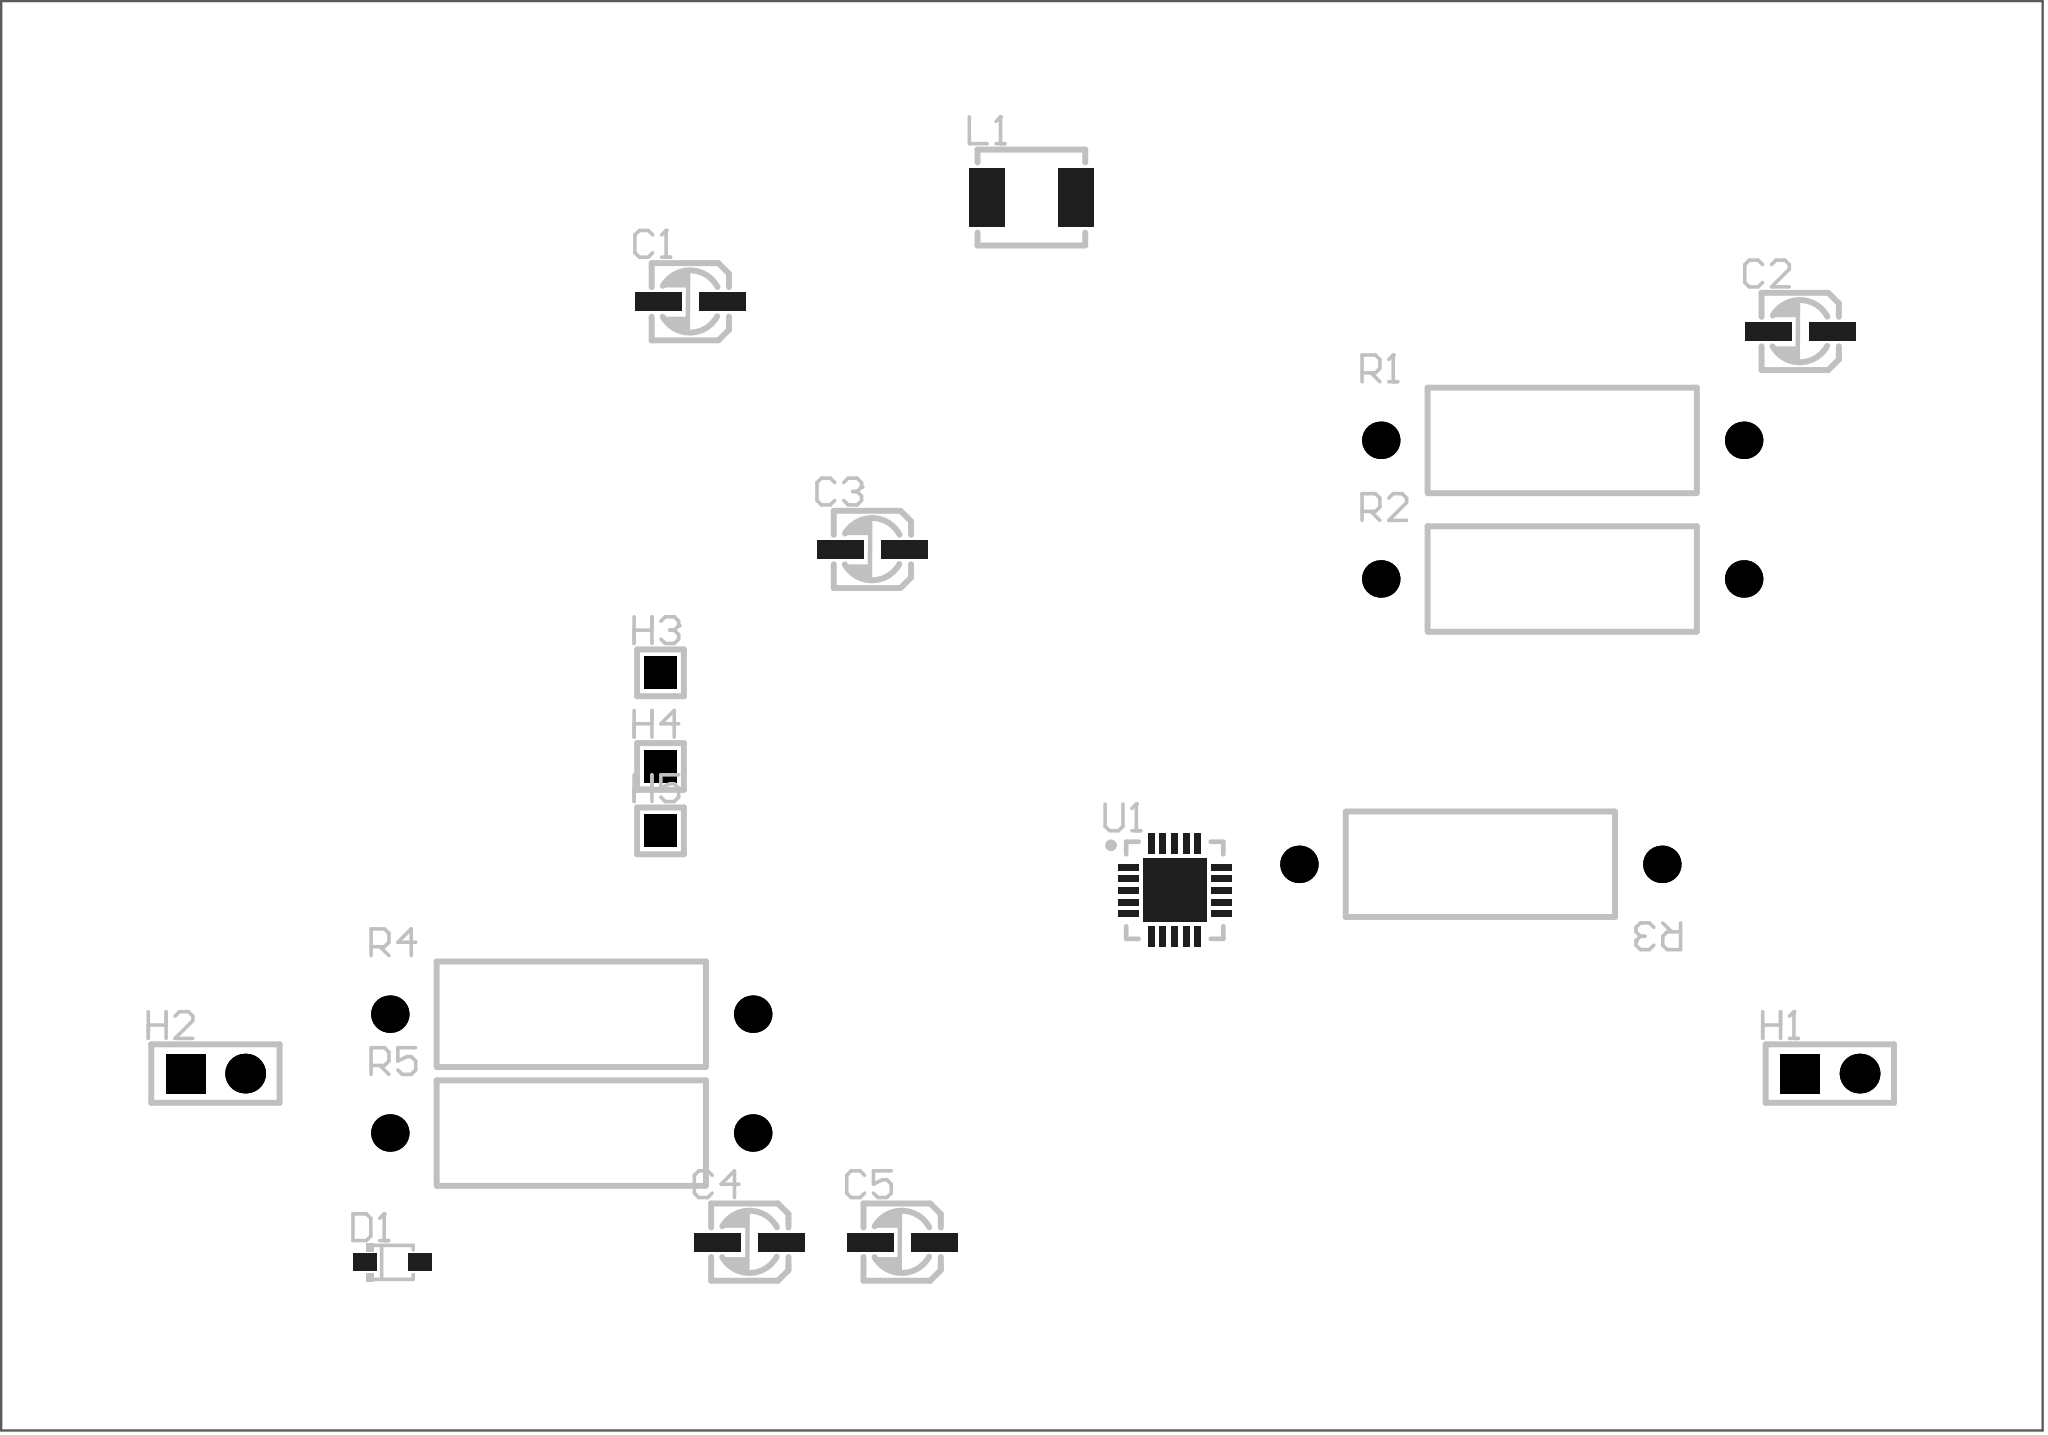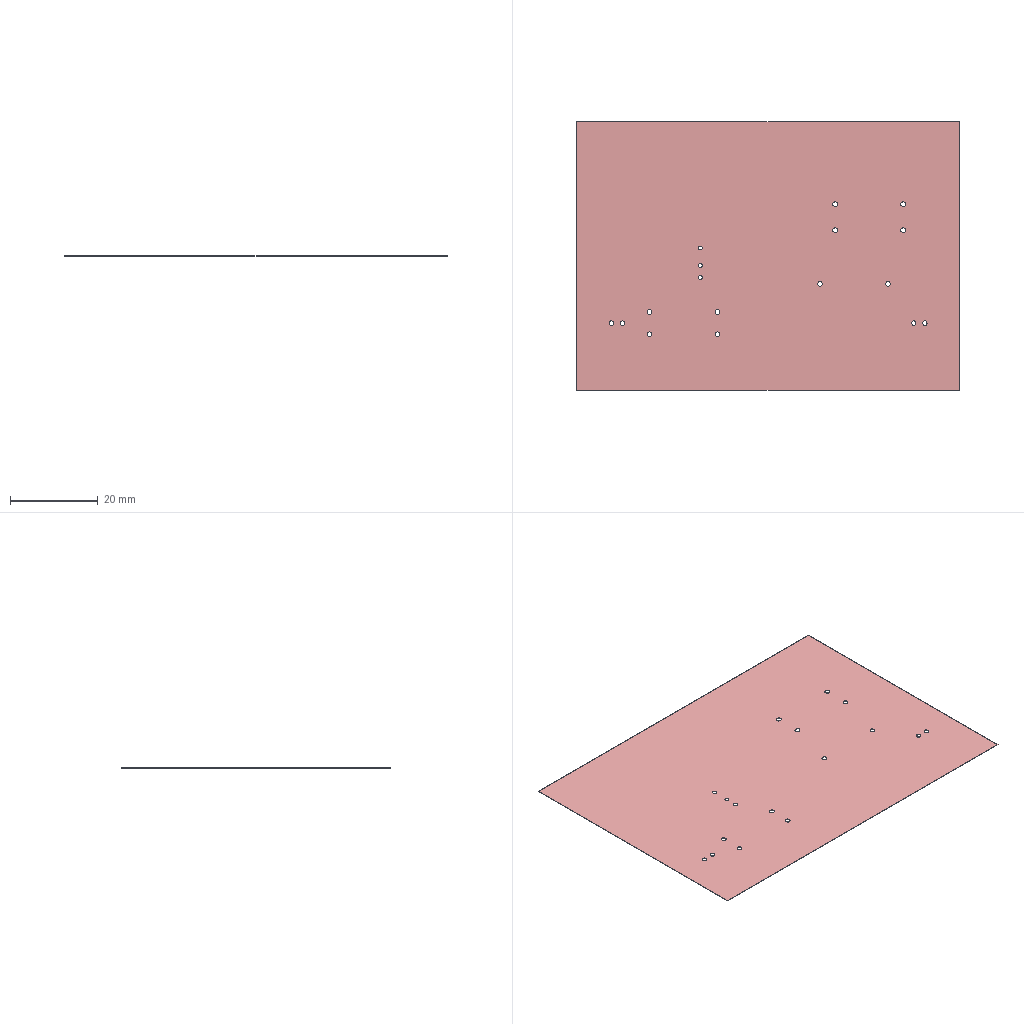Circuit board layout | Altium Designer | box 87.2 x 61.1 x 0.1 mm
Layer stack:
# Altium Designer layer stack of  (unit mm; dielectric type: 0 none, 1 core, 2 prepreg, 3 surface material)
index,name,kind,layer,copper_thickness_mm,dielectric_type,dielectric_thickness_mm,dielectric_material,dielectric_constant
0,Top Paste Mask Layer,other,,,,,,
1,Top Silkscreen Layer,other,,,,,,
2,Top Solder Mask Layer,dielectric,,,3,0.01,,3.3
3,Top Layer,copper,Top Layer,0.035,,,,
4,Bottom Layer,copper,Bottom Layer,0.035,,,,
5,Bottom Solder Mask Layer,dielectric,,,3,0.01,,3.3
6,Bottom Silkscreen Layer,other,,,,,,
7,Bottom Paste Mask Layer,other,,,,,,
# drill layer pairs: low layer,high layer
drill_pair,Top Layer,Bottom Layer
Part placement:
Designator,Comment,Layer,Footprint,Center-X(mm),Center-Y(mm),Rotation
C1,0.1uF,TopLayer,C_Ele_SMD_3x5.4mm,99.284,118.106,0
C2,100nF/250V,TopLayer,C_Ele_SMD_3x5.4mm,146.689,116.835,0
C3,0.1u,TopLayer,C_Ele_SMD_3x5.4mm,107.062,107.515,0
C4,10nF,TopLayer,C_Ele_SMD_3x5.4mm,101.825,77.899,0
C5,10nF,TopLayer,C_Ele_SMD_3x5.4mm,108.332,77.899,0
D1,BAT165E6327,TopLayer,SOD-323_L1.8-W1.3-LS2.5-RD,86.547,77.038,0
H1,,TopLayer,HDR-TH_2P-P2.54-V-F,147.954,85.11,0
H2,,TopLayer,HDR-TH_2P-P2.54-V-F,79,85.11,0
H3,,TopLayer,HDR-TH_1P-V-M_XKB_X4611WV-01I-C28D40,98.01,102.244,0
H4,,TopLayer,HDR-TH_1P-V-M_XKB_X4611WV-01I-C28D40,98.01,98.24,0
H5,,TopLayer,HDR-TH_1P-V-M_XKB_X4611WV-01I-C28D40,98.01,95.486,0
L1,4.7uH,TopLayer,IND-SMD_L4.6-W4.1-A,113.85,122.566,0
R1,1.72M,TopLayer,Res_1W,136.524,112.186,0
R2,15k,TopLayer,Res_1W,136.524,106.259,0
R3,18k,TopLayer,Res_1W,133.029,94.056,180
R4,1k,TopLayer,Res_1W,94.2,87.65,0
R5,1k,TopLayer,Res_1W,94.2,82.57,0
U1,DRV2700,TopLayer,TI-RGP20-2700X2700TP_V,119.974,92.946,0
Pad and via stacks:
# Altium Designer via and pad stacks of  (unit mm). Each distinct definition once, with the count of objects using it.
# via: kind,start_layer,end_layer,hole_mm,diameter_mm,mode(0 simple;1 top-mid-bottom;2 full stack),diameter_per_layer,count,example_net
# pad: kind,layer,hole_mm,hole_type(0 round;1 square;2 slot),plating,top_size,top_shape(1 round;2 rect;3 octagon;9 rounded rect),mid_size,bottom_size,mode,footprint,size_per_layer,count,example
pad,Top Layer,0,0,plated,1.999x0.8001,2,1.999x0.8001,1.999x0.8001,0,C_Ele_SMD_3x5.4mm,,10,C1.1
pad,Top Layer,0,0,plated,1x0.75,2,1x0.75,1x0.75,0,SOD-323_L1.8-W1.3-LS2.5-RD,,2,D1.2
pad,Top Layer,0,0,plated,2.5x1.5,2,2.5x1.5,2.5x1.5,0,IND-SMD_L4.6-W4.1-A,,2,L1.1
pad,Top Layer,0,0,plated,2.705x2.705,2,2.705x2.705,2.705x2.705,0,TI-RGP20-2700X2700TP_V,,1,U1.21
pad,Top Layer,0,0,plated,0.2921x0.8763,2,0.2921x0.8763,0.2921x0.8763,0,TI-RGP20-2700X2700TP_V,,20,U1.20
pad,Multi-Layer,1,0,plated,1.7x1.7,2,1.7x1.7,1.7x1.7,0,HDR-TH_2P-P2.54-V-F,,2,H1.1
pad,Multi-Layer,1,0,plated,1.7x1.7,1,1.7x1.7,1.7x1.7,0,HDR-TH_2P-P2.54-V-F,,2,H1.2
pad,Multi-Layer,0.9,0,plated,1.4x1.4,2,1.4x1.4,1.4x1.4,0,HDR-TH_1P-V-M_XKB_X4611WV-01I-C28D40,,3,H3.1
pad,Multi-Layer,1.1,0,plated,1.6x1.6,1,1.6x1.6,1.6x1.6,0,Res_1W,,10,R1.1
via,Top Layer,Bottom Layer,0.2997,0.5004,0,,9,GND
Design rules, without the lines most boards share:
# Altium Designer design rules of  (exported by Altium Designer, unit mm)
# columns: name | kind | enabled | priority | scope1 | scope2 | descriptor | typed fields (field=value)
Plane_innerPlane | 0 | disabled | 1 | All | All | Clearance Constraint (Gap=6mil) (Disabled)(All),(All) | gap=0.1524
Plane_innerPlane_1 | 63 | disabled | 1 | All | All | Board Clearance Constraint (Gap=0mil) (Disabled)(All) |
Copper_copperRegion | 0 | disabled | 2 | All | All | Clearance Constraint (Gap=6mil) (Disabled)(All),(All) | gap=0.1524
Copper_copperRegion_1 | 63 | disabled | 2 | All | All | Board Clearance Constraint (Gap=0mil) (Disabled)(All) |
copperThickness1oz | 0 | enabled | 3 | All | All | Clearance Constraint (Gap=6mil) (All),(All) | gap=0.1524
copperThickness1oz_1 | 63 | enabled | 3 | All | All | Board Clearance Constraint (Gap=0mil) (All) |
otherClearance | 52 | enabled | 1 | All | All | Hole To Hole Clearance (Gap=11.8mil) (All),(All) | gap=0.2997
copperThickness1oz_2 | 2 | enabled | 1 | All | All | Width Constraint (Min=5mil) (Max=100mil) (Preferred=10mil) (All) |
differentialPair | 51 | enabled | 1 | All | All | Differential Pairs Uncoupled Length using the Gap Constraints (Min=5mil) (Max=6mil) (Prefered=6mil)  and Width Constraints (Min=5mil) (Max=100mil) (Prefered=100mil) (All) |
viaSize | 11 | enabled | 1 | All | All | Routing Via (MinHoleWidth=19.7mil) (MaxHoleWidth=393.7mil) (PreferredHoleWidth=24mil) (MinWidth=11.8mil) (MaxWidth=248mil) (PreferedWidth=12mil) (All) | via_min_hole=0.5004 via_max_hole=10 via_preferred_diameter=0.3048 via_preferred_hole=0.6096